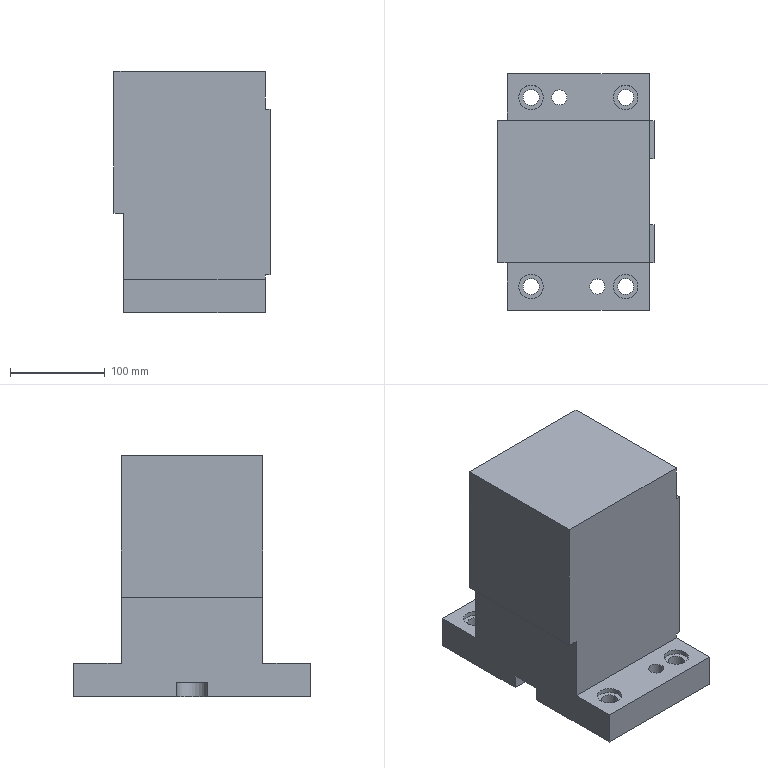Part | NX | features solid 2 | 1 solid | 44 faces | box 165 x 250 x 255 mm | volume 5111238 mm3 | plane 33 | cylinder 11 | commonest cylinder face diameters 17 x4 26 x4 16 x2 32 x1
STEP:
#1=CARTESIAN_POINT('',(655.,586.5,-210.));
#2=VERTEX_POINT('',#1);
#3=CARTESIAN_POINT('',(655.,595.,-210.));
#4=DIRECTION('',(0.,0.,1.));
#5=DIRECTION('',(0.,-1.,0.));
#6=AXIS2_PLACEMENT_3D('',#3,#4,#5);
#7=CIRCLE('',#6,8.5);
#8=EDGE_CURVE('',#2,#2,#7,.T.);
#9=ORIENTED_EDGE('',*,*,#8,.T.);
#10=EDGE_LOOP('',(#9));
#11=FACE_BOUND('',#10,.T.);
#12=CARTESIAN_POINT('',(655.,786.5,-210.));
#13=VERTEX_POINT('',#12);
#14=CARTESIAN_POINT('',(655.,795.,-210.));
#15=DIRECTION('',(0.,0.,1.));
#16=DIRECTION('',(0.,-1.,0.));
#17=AXIS2_PLACEMENT_3D('',#14,#15,#16);
#18=CIRCLE('',#17,8.5);
#19=EDGE_CURVE('',#13,#13,#18,.T.);
#20=ORIENTED_EDGE('',*,*,#19,.T.);
#21=EDGE_LOOP('',(#20));
#22=FACE_BOUND('',#21,.T.);
#23=CARTESIAN_POINT('',(685.,787.,-210.));
#24=VERTEX_POINT('',#23);
#25=CARTESIAN_POINT('',(685.,795.,-210.));
#26=DIRECTION('',(0.,0.,1.));
#27=DIRECTION('',(0.,-1.,0.));
#28=AXIS2_PLACEMENT_3D('',#25,#26,#27);
#29=CIRCLE('',#28,8.);
#30=EDGE_CURVE('',#24,#24,#29,.T.);
#31=ORIENTED_EDGE('',*,*,#30,.T.);
#32=EDGE_LOOP('',(#31));
#33=FACE_BOUND('',#32,.T.);
#34=CARTESIAN_POINT('',(755.,786.5,-210.));
#35=VERTEX_POINT('',#34);
#36=CARTESIAN_POINT('',(755.,795.,-210.));
#37=DIRECTION('',(0.,0.,1.));
#38=DIRECTION('',(0.,-1.,0.));
#39=AXIS2_PLACEMENT_3D('',#36,#37,#38);
#40=CIRCLE('',#39,8.5);
#41=EDGE_CURVE('',#35,#35,#40,.T.);
#42=ORIENTED_EDGE('',*,*,#41,.T.);
#43=EDGE_LOOP('',(#42));
#44=FACE_BOUND('',#43,.T.);
#45=CARTESIAN_POINT('',(725.,587.,-210.));
#46=VERTEX_POINT('',#45);
#47=CARTESIAN_POINT('',(725.,595.,-210.));
#48=DIRECTION('',(0.,0.,1.));
#49=DIRECTION('',(0.,-1.,0.));
#50=AXIS2_PLACEMENT_3D('',#47,#48,#49);
#51=CIRCLE('',#50,8.);
#52=EDGE_CURVE('',#46,#46,#51,.T.);
#53=ORIENTED_EDGE('',*,*,#52,.T.);
#54=EDGE_LOOP('',(#53));
#55=FACE_BOUND('',#54,.T.);
#56=CARTESIAN_POINT('',(755.,586.5,-210.));
#57=VERTEX_POINT('',#56);
#58=CARTESIAN_POINT('',(755.,595.,-210.));
#59=DIRECTION('',(0.,0.,1.));
#60=DIRECTION('',(0.,-1.,0.));
#61=AXIS2_PLACEMENT_3D('',#58,#59,#60);
#62=CIRCLE('',#61,8.5);
#63=EDGE_CURVE('',#57,#57,#62,.T.);
#64=ORIENTED_EDGE('',*,*,#63,.T.);
#65=EDGE_LOOP('',(#64));
#66=FACE_BOUND('',#65,.T.);
#67=CARTESIAN_POINT('',(714.,679.031,-210.));
#68=VERTEX_POINT('',#67);
#69=CARTESIAN_POINT('',(714.,679.,-210.));
#70=VERTEX_POINT('',#69);
#71=CARTESIAN_POINT('',(714.,810.,-210.));
#72=DIRECTION('',(0.,-1.,0.));
#73=VECTOR('',#72,1000.);
#74=LINE('',#71,#73);
#75=EDGE_CURVE('',#68,#70,#74,.T.);
#76=ORIENTED_EDGE('',*,*,#75,.F.);
#77=CARTESIAN_POINT('',(714.,710.969,-210.));
#78=VERTEX_POINT('',#77);
#79=CARTESIAN_POINT('',(715.,695.,-210.));
#80=DIRECTION('',(0.,0.,-1.));
#81=DIRECTION('',(-1.,0.,0.));
#82=AXIS2_PLACEMENT_3D('',#79,#80,#81);
#83=CIRCLE('',#82,16.);
#84=EDGE_CURVE('',#68,#78,#83,.F.);
#85=ORIENTED_EDGE('',*,*,#84,.T.);
#86=CARTESIAN_POINT('',(714.,711.,-210.));
#87=VERTEX_POINT('',#86);
#88=CARTESIAN_POINT('',(714.,810.,-210.));
#89=DIRECTION('',(0.,-1.,0.));
#90=VECTOR('',#89,1000.);
#91=LINE('',#88,#90);
#92=EDGE_CURVE('',#87,#78,#91,.T.);
#93=ORIENTED_EDGE('',*,*,#92,.F.);
#94=CARTESIAN_POINT('',(630.,711.,-210.));
#95=VERTEX_POINT('',#94);
#96=CARTESIAN_POINT('',(780.,711.,-210.));
#97=DIRECTION('',(-1.,0.,0.));
#98=VECTOR('',#97,1000.);
#99=LINE('',#96,#98);
#100=EDGE_CURVE('',#87,#95,#99,.T.);
#101=ORIENTED_EDGE('',*,*,#100,.T.);
#102=CARTESIAN_POINT('',(630.,820.,-210.));
#103=VERTEX_POINT('',#102);
#104=CARTESIAN_POINT('',(630.,810.,-210.));
#105=DIRECTION('',(0.,1.,0.));
#106=VECTOR('',#105,1000.);
#107=LINE('',#104,#106);
#108=EDGE_CURVE('',#103,#95,#107,.F.);
#109=ORIENTED_EDGE('',*,*,#108,.F.);
#110=CARTESIAN_POINT('',(780.,820.,-210.));
#111=VERTEX_POINT('',#110);
#112=CARTESIAN_POINT('',(780.,820.,-210.));
#113=DIRECTION('',(1.,0.,0.));
#114=VECTOR('',#113,1000.);
#115=LINE('',#112,#114);
#116=EDGE_CURVE('',#111,#103,#115,.F.);
#117=ORIENTED_EDGE('',*,*,#116,.F.);
#118=CARTESIAN_POINT('',(780.,570.,-210.));
#119=VERTEX_POINT('',#118);
#120=CARTESIAN_POINT('',(780.,810.,-210.));
#121=DIRECTION('',(0.,-1.,0.));
#122=VECTOR('',#121,1000.);
#123=LINE('',#120,#122);
#124=EDGE_CURVE('',#111,#119,#123,.T.);
#125=ORIENTED_EDGE('',*,*,#124,.T.);
#126=CARTESIAN_POINT('',(630.,570.,-210.));
#127=VERTEX_POINT('',#126);
#128=CARTESIAN_POINT('',(780.,570.,-210.));
#129=DIRECTION('',(1.,0.,0.));
#130=VECTOR('',#129,1000.);
#131=LINE('',#128,#130);
#132=EDGE_CURVE('',#119,#127,#131,.F.);
#133=ORIENTED_EDGE('',*,*,#132,.T.);
#134=CARTESIAN_POINT('',(630.,679.,-210.));
#135=VERTEX_POINT('',#134);
#136=CARTESIAN_POINT('',(630.,810.,-210.));
#137=DIRECTION('',(0.,1.,0.));
#138=VECTOR('',#137,1000.);
#139=LINE('',#136,#138);
#140=EDGE_CURVE('',#135,#127,#139,.F.);
#141=ORIENTED_EDGE('',*,*,#140,.F.);
#142=CARTESIAN_POINT('',(780.,679.,-210.));
#143=DIRECTION('',(1.,0.,0.));
#144=VECTOR('',#143,1000.);
#145=LINE('',#142,#144);
#146=EDGE_CURVE('',#135,#70,#145,.T.);
#147=ORIENTED_EDGE('',*,*,#146,.T.);
#148=EDGE_LOOP('',(#76,#85,#93,#101,#109,#117,#125,#133,#141,#147));
#149=FACE_BOUND('',#148,.T.);
#150=CARTESIAN_POINT('',(780.,810.,-210.));
#151=DIRECTION('',(0.,0.,-1.));
#152=DIRECTION('',(0.,1.,0.));
#153=AXIS2_PLACEMENT_3D('',#150,#151,#152);
#154=PLANE('',#153);
#155=ADVANCED_FACE('',(#11,#22,#33,#44,#55,#66,#149),#154,.T.);
#156=CARTESIAN_POINT('',(714.,679.031,-195.));
#157=VERTEX_POINT('',#156);
#158=CARTESIAN_POINT('',(714.,679.031,-195.));
#159=DIRECTION('',(0.,0.,-1.));
#160=VECTOR('',#159,1000.);
#161=LINE('',#158,#160);
#162=EDGE_CURVE('',#68,#157,#161,.F.);
#163=ORIENTED_EDGE('',*,*,#162,.F.);
#164=ORIENTED_EDGE('',*,*,#75,.T.);
#165=CARTESIAN_POINT('',(714.,679.,-195.));
#166=VERTEX_POINT('',#165);
#167=CARTESIAN_POINT('',(714.,679.,-195.));
#168=DIRECTION('',(0.,0.,-1.));
#169=VECTOR('',#168,1000.);
#170=LINE('',#167,#169);
#171=EDGE_CURVE('',#166,#70,#170,.T.);
#172=ORIENTED_EDGE('',*,*,#171,.F.);
#173=CARTESIAN_POINT('',(714.,650.,-195.));
#174=DIRECTION('',(0.,-1.,0.));
#175=VECTOR('',#174,1000.);
#176=LINE('',#173,#175);
#177=EDGE_CURVE('',#157,#166,#176,.T.);
#178=ORIENTED_EDGE('',*,*,#177,.F.);
#179=EDGE_LOOP('',(#163,#164,#172,#178));
#180=FACE_BOUND('',#179,.T.);
#181=CARTESIAN_POINT('',(714.,810.,-180.));
#182=DIRECTION('',(1.,0.,0.));
#183=DIRECTION('',(0.,0.,-1.));
#184=AXIS2_PLACEMENT_3D('',#181,#182,#183);
#185=PLANE('',#184);
#186=ADVANCED_FACE('',(#180),#185,.F.);
#187=CARTESIAN_POINT('',(714.,710.969,-195.));
#188=VERTEX_POINT('',#187);
#189=CARTESIAN_POINT('',(714.,710.969,-195.));
#190=DIRECTION('',(0.,0.,-1.));
#191=VECTOR('',#190,1000.);
#192=LINE('',#189,#191);
#193=EDGE_CURVE('',#188,#78,#192,.T.);
#194=ORIENTED_EDGE('',*,*,#193,.F.);
#195=CARTESIAN_POINT('',(714.,711.,-195.));
#196=VERTEX_POINT('',#195);
#197=CARTESIAN_POINT('',(714.,650.,-195.));
#198=DIRECTION('',(0.,-1.,0.));
#199=VECTOR('',#198,1000.);
#200=LINE('',#197,#199);
#201=EDGE_CURVE('',#196,#188,#200,.T.);
#202=ORIENTED_EDGE('',*,*,#201,.F.);
#203=CARTESIAN_POINT('',(714.,711.,-180.));
#204=DIRECTION('',(0.,0.,-1.));
#205=VECTOR('',#204,1000.);
#206=LINE('',#203,#205);
#207=EDGE_CURVE('',#196,#87,#206,.T.);
#208=ORIENTED_EDGE('',*,*,#207,.T.);
#209=ORIENTED_EDGE('',*,*,#92,.T.);
#210=EDGE_LOOP('',(#194,#202,#208,#209));
#211=FACE_BOUND('',#210,.T.);
#212=CARTESIAN_POINT('',(714.,810.,-180.));
#213=DIRECTION('',(1.,0.,0.));
#214=DIRECTION('',(0.,0.,-1.));
#215=AXIS2_PLACEMENT_3D('',#212,#213,#214);
#216=PLANE('',#215);
#217=ADVANCED_FACE('',(#211),#216,.F.);
#218=CARTESIAN_POINT('',(715.,695.,-195.));
#219=DIRECTION('',(0.,0.,-1.));
#220=DIRECTION('',(-1.,0.,0.));
#221=AXIS2_PLACEMENT_3D('',#218,#219,#220);
#222=CIRCLE('',#221,16.);
#223=EDGE_CURVE('',#157,#188,#222,.F.);
#224=ORIENTED_EDGE('',*,*,#223,.F.);
#225=ORIENTED_EDGE('',*,*,#177,.T.);
#226=CARTESIAN_POINT('',(630.,679.,-195.));
#227=VERTEX_POINT('',#226);
#228=CARTESIAN_POINT('',(740.,679.,-195.));
#229=DIRECTION('',(-1.,0.,0.));
#230=VECTOR('',#229,1000.);
#231=LINE('',#228,#230);
#232=EDGE_CURVE('',#227,#166,#231,.F.);
#233=ORIENTED_EDGE('',*,*,#232,.F.);
#234=CARTESIAN_POINT('',(630.,711.,-195.));
#235=VERTEX_POINT('',#234);
#236=CARTESIAN_POINT('',(630.,810.,-195.));
#237=DIRECTION('',(0.,1.,0.));
#238=VECTOR('',#237,1000.);
#239=LINE('',#236,#238);
#240=EDGE_CURVE('',#235,#227,#239,.F.);
#241=ORIENTED_EDGE('',*,*,#240,.F.);
#242=CARTESIAN_POINT('',(740.,711.,-195.));
#243=DIRECTION('',(1.,0.,0.));
#244=VECTOR('',#243,1000.);
#245=LINE('',#242,#244);
#246=EDGE_CURVE('',#196,#235,#245,.F.);
#247=ORIENTED_EDGE('',*,*,#246,.F.);
#248=ORIENTED_EDGE('',*,*,#201,.T.);
#249=EDGE_LOOP('',(#224,#225,#233,#241,#247,#248));
#250=FACE_BOUND('',#249,.T.);
#251=CARTESIAN_POINT('',(740.,650.,-195.));
#252=DIRECTION('',(0.,0.,-1.));
#253=DIRECTION('',(-1.,0.,0.));
#254=AXIS2_PLACEMENT_3D('',#251,#252,#253);
#255=PLANE('',#254);
#256=ADVANCED_FACE('',(#250),#255,.T.);
#257=CARTESIAN_POINT('',(780.,730.,5.));
#258=VERTEX_POINT('',#257);
#259=CARTESIAN_POINT('',(780.,770.,5.));
#260=VERTEX_POINT('',#259);
#261=CARTESIAN_POINT('',(780.,730.,5.));
#262=DIRECTION('',(0.,1.,0.));
#263=VECTOR('',#262,1000.);
#264=LINE('',#261,#263);
#265=EDGE_CURVE('',#258,#260,#264,.T.);
#266=ORIENTED_EDGE('',*,*,#265,.T.);
#267=CARTESIAN_POINT('',(780.,770.,45.));
#268=VERTEX_POINT('',#267);
#269=CARTESIAN_POINT('',(780.,770.,-220.));
#270=DIRECTION('',(0.,0.,-1.));
#271=VECTOR('',#270,1000.);
#272=LINE('',#269,#271);
#273=EDGE_CURVE('',#260,#268,#272,.F.);
#274=ORIENTED_EDGE('',*,*,#273,.T.);
#275=CARTESIAN_POINT('',(780.,620.,45.));
#276=VERTEX_POINT('',#275);
#277=CARTESIAN_POINT('',(780.,810.,45.));
#278=DIRECTION('',(0.,-1.,0.));
#279=VECTOR('',#278,1000.);
#280=LINE('',#277,#279);
#281=EDGE_CURVE('',#268,#276,#280,.T.);
#282=ORIENTED_EDGE('',*,*,#281,.T.);
#283=CARTESIAN_POINT('',(780.,620.,5.));
#284=VERTEX_POINT('',#283);
#285=CARTESIAN_POINT('',(780.,620.,-220.));
#286=DIRECTION('',(0.,0.,1.));
#287=VECTOR('',#286,1000.);
#288=LINE('',#285,#287);
#289=EDGE_CURVE('',#284,#276,#288,.T.);
#290=ORIENTED_EDGE('',*,*,#289,.F.);
#291=CARTESIAN_POINT('',(780.,660.,5.));
#292=VERTEX_POINT('',#291);
#293=CARTESIAN_POINT('',(780.,620.,5.));
#294=DIRECTION('',(0.,1.,0.));
#295=VECTOR('',#294,1000.);
#296=LINE('',#293,#295);
#297=EDGE_CURVE('',#284,#292,#296,.T.);
#298=ORIENTED_EDGE('',*,*,#297,.T.);
#299=CARTESIAN_POINT('',(780.,810.,5.));
#300=DIRECTION('',(0.,-1.,0.));
#301=VECTOR('',#300,1000.);
#302=LINE('',#299,#301);
#303=EDGE_CURVE('',#258,#292,#302,.T.);
#304=ORIENTED_EDGE('',*,*,#303,.F.);
#305=EDGE_LOOP('',(#266,#274,#282,#290,#298,#304));
#306=FACE_BOUND('',#305,.T.);
#307=CARTESIAN_POINT('',(780.,810.,-220.));
#308=DIRECTION('',(1.,0.,0.));
#309=DIRECTION('',(0.,-1.,0.));
#310=AXIS2_PLACEMENT_3D('',#307,#308,#309);
#311=PLANE('',#310);
#312=ADVANCED_FACE('',(#306),#311,.T.);
#313=ORIENTED_EDGE('',*,*,#108,.T.);
#314=CARTESIAN_POINT('',(630.,711.,-220.));
#315=DIRECTION('',(0.,0.,-1.));
#316=VECTOR('',#315,1000.);
#317=LINE('',#314,#316);
#318=EDGE_CURVE('',#95,#235,#317,.F.);
#319=ORIENTED_EDGE('',*,*,#318,.T.);
#320=ORIENTED_EDGE('',*,*,#240,.T.);
#321=CARTESIAN_POINT('',(630.,679.,-220.));
#322=DIRECTION('',(0.,0.,1.));
#323=VECTOR('',#322,1000.);
#324=LINE('',#321,#323);
#325=EDGE_CURVE('',#227,#135,#324,.F.);
#326=ORIENTED_EDGE('',*,*,#325,.T.);
#327=ORIENTED_EDGE('',*,*,#140,.T.);
#328=CARTESIAN_POINT('',(630.,570.,-175.));
#329=VERTEX_POINT('',#328);
#330=CARTESIAN_POINT('',(630.,570.,-180.));
#331=DIRECTION('',(0.,0.,-1.));
#332=VECTOR('',#331,1000.);
#333=LINE('',#330,#332);
#334=EDGE_CURVE('',#329,#127,#333,.T.);
#335=ORIENTED_EDGE('',*,*,#334,.F.);
#336=CARTESIAN_POINT('',(630.,620.,-175.));
#337=VERTEX_POINT('',#336);
#338=CARTESIAN_POINT('',(630.,810.,-175.));
#339=DIRECTION('',(0.,-1.,0.));
#340=VECTOR('',#339,1000.);
#341=LINE('',#338,#340);
#342=EDGE_CURVE('',#337,#329,#341,.T.);
#343=ORIENTED_EDGE('',*,*,#342,.F.);
#344=CARTESIAN_POINT('',(630.,620.,-105.));
#345=VERTEX_POINT('',#344);
#346=CARTESIAN_POINT('',(630.,620.,-220.));
#347=DIRECTION('',(0.,0.,-1.));
#348=VECTOR('',#347,1000.);
#349=LINE('',#346,#348);
#350=EDGE_CURVE('',#337,#345,#349,.F.);
#351=ORIENTED_EDGE('',*,*,#350,.T.);
#352=CARTESIAN_POINT('',(630.,770.,-105.));
#353=VERTEX_POINT('',#352);
#354=CARTESIAN_POINT('',(630.,770.,-105.));
#355=DIRECTION('',(0.,1.,0.));
#356=VECTOR('',#355,1000.);
#357=LINE('',#354,#356);
#358=EDGE_CURVE('',#353,#345,#357,.F.);
#359=ORIENTED_EDGE('',*,*,#358,.F.);
#360=CARTESIAN_POINT('',(630.,770.,-175.));
#361=VERTEX_POINT('',#360);
#362=CARTESIAN_POINT('',(630.,770.,-220.));
#363=DIRECTION('',(0.,0.,1.));
#364=VECTOR('',#363,1000.);
#365=LINE('',#362,#364);
#366=EDGE_CURVE('',#361,#353,#365,.T.);
#367=ORIENTED_EDGE('',*,*,#366,.F.);
#368=CARTESIAN_POINT('',(630.,820.,-175.));
#369=VERTEX_POINT('',#368);
#370=CARTESIAN_POINT('',(630.,810.,-175.));
#371=DIRECTION('',(0.,-1.,0.));
#372=VECTOR('',#371,1000.);
#373=LINE('',#370,#372);
#374=EDGE_CURVE('',#361,#369,#373,.F.);
#375=ORIENTED_EDGE('',*,*,#374,.T.);
#376=CARTESIAN_POINT('',(630.,820.,-180.));
#377=DIRECTION('',(0.,0.,-1.));
#378=VECTOR('',#377,1000.);
#379=LINE('',#376,#378);
#380=EDGE_CURVE('',#369,#103,#379,.T.);
#381=ORIENTED_EDGE('',*,*,#380,.T.);
#382=EDGE_LOOP('',(#313,#319,#320,#326,#327,#335,#343,#351,#359,#367,#375,#381));
#383=FACE_BOUND('',#382,.T.);
#384=CARTESIAN_POINT('',(630.,810.,-220.));
#385=DIRECTION('',(1.,0.,0.));
#386=DIRECTION('',(0.,-1.,0.));
#387=AXIS2_PLACEMENT_3D('',#384,#385,#386);
#388=PLANE('',#387);
#389=ADVANCED_FACE('',(#383),#388,.F.);
#390=CARTESIAN_POINT('',(780.,730.,-170.));
#391=VERTEX_POINT('',#390);
#392=CARTESIAN_POINT('',(780.,770.,-170.));
#393=VERTEX_POINT('',#392);
#394=CARTESIAN_POINT('',(780.,730.,-170.));
#395=DIRECTION('',(0.,1.,0.));
#396=VECTOR('',#395,1000.);
#397=LINE('',#394,#396);
#398=EDGE_CURVE('',#391,#393,#397,.T.);
#399=ORIENTED_EDGE('',*,*,#398,.F.);
#400=CARTESIAN_POINT('',(780.,660.,-170.));
#401=VERTEX_POINT('',#400);
#402=CARTESIAN_POINT('',(780.,810.,-170.));
#403=DIRECTION('',(0.,-1.,0.));
#404=VECTOR('',#403,1000.);
#405=LINE('',#402,#404);
#406=EDGE_CURVE('',#391,#401,#405,.T.);
#407=ORIENTED_EDGE('',*,*,#406,.T.);
#408=CARTESIAN_POINT('',(780.,620.,-170.));
#409=VERTEX_POINT('',#408);
#410=CARTESIAN_POINT('',(780.,620.,-170.));
#411=DIRECTION('',(0.,1.,0.));
#412=VECTOR('',#411,1000.);
#413=LINE('',#410,#412);
#414=EDGE_CURVE('',#409,#401,#413,.T.);
#415=ORIENTED_EDGE('',*,*,#414,.F.);
#416=CARTESIAN_POINT('',(780.,620.,-175.));
#417=VERTEX_POINT('',#416);
#418=CARTESIAN_POINT('',(780.,620.,-220.));
#419=DIRECTION('',(0.,0.,1.));
#420=VECTOR('',#419,1000.);
#421=LINE('',#418,#420);
#422=EDGE_CURVE('',#417,#409,#421,.T.);
#423=ORIENTED_EDGE('',*,*,#422,.F.);
#424=CARTESIAN_POINT('',(780.,570.,-175.));
#425=VERTEX_POINT('',#424);
#426=CARTESIAN_POINT('',(780.,620.,-175.));
#427=DIRECTION('',(0.,1.,0.));
#428=VECTOR('',#427,1000.);
#429=LINE('',#426,#428);
#430=EDGE_CURVE('',#417,#425,#429,.F.);
#431=ORIENTED_EDGE('',*,*,#430,.T.);
#432=CARTESIAN_POINT('',(780.,570.,-180.));
#433=DIRECTION('',(0.,0.,-1.));
#434=VECTOR('',#433,1000.);
#435=LINE('',#432,#434);
#436=EDGE_CURVE('',#425,#119,#435,.T.);
#437=ORIENTED_EDGE('',*,*,#436,.T.);
#438=ORIENTED_EDGE('',*,*,#124,.F.);
#439=CARTESIAN_POINT('',(780.,820.,-175.));
#440=VERTEX_POINT('',#439);
#441=CARTESIAN_POINT('',(780.,820.,-180.));
#442=DIRECTION('',(0.,0.,1.));
#443=VECTOR('',#442,1000.);
#444=LINE('',#441,#443);
#445=EDGE_CURVE('',#440,#111,#444,.F.);
#446=ORIENTED_EDGE('',*,*,#445,.F.);
#447=CARTESIAN_POINT('',(780.,770.,-175.));
#448=VERTEX_POINT('',#447);
#449=CARTESIAN_POINT('',(780.,770.,-175.));
#450=DIRECTION('',(0.,1.,0.));
#451=VECTOR('',#450,1000.);
#452=LINE('',#449,#451);
#453=EDGE_CURVE('',#448,#440,#452,.T.);
#454=ORIENTED_EDGE('',*,*,#453,.F.);
#455=CARTESIAN_POINT('',(780.,770.,-220.));
#456=DIRECTION('',(0.,0.,-1.));
#457=VECTOR('',#456,1000.);
#458=LINE('',#455,#457);
#459=EDGE_CURVE('',#448,#393,#458,.F.);
#460=ORIENTED_EDGE('',*,*,#459,.T.);
#461=EDGE_LOOP('',(#399,#407,#415,#423,#431,#437,#438,#446,#454,#460));
#462=FACE_BOUND('',#461,.T.);
#463=CARTESIAN_POINT('',(780.,810.,-220.));
#464=DIRECTION('',(1.,0.,0.));
#465=DIRECTION('',(0.,-1.,0.));
#466=AXIS2_PLACEMENT_3D('',#463,#464,#465);
#467=PLANE('',#466);
#468=ADVANCED_FACE('',(#462),#467,.T.);
#469=ORIENTED_EDGE('',*,*,#459,.F.);
#470=CARTESIAN_POINT('',(780.,770.,-175.));
#471=DIRECTION('',(1.,0.,0.));
#472=VECTOR('',#471,1000.);
#473=LINE('',#470,#472);
#474=EDGE_CURVE('',#448,#361,#473,.F.);
#475=ORIENTED_EDGE('',*,*,#474,.T.);
#476=ORIENTED_EDGE('',*,*,#366,.T.);
#477=CARTESIAN_POINT('',(620.,770.,-105.));
#478=VERTEX_POINT('',#477);
#479=CARTESIAN_POINT('',(630.,770.,-105.));
#480=DIRECTION('',(1.,0.,0.));
#481=VECTOR('',#480,1000.);
#482=LINE('',#479,#481);
#483=EDGE_CURVE('',#353,#478,#482,.F.);
#484=ORIENTED_EDGE('',*,*,#483,.T.);
#485=CARTESIAN_POINT('',(620.,770.,45.));
#486=VERTEX_POINT('',#485);
#487=CARTESIAN_POINT('',(620.,770.,45.));
#488=DIRECTION('',(0.,0.,1.));
#489=VECTOR('',#488,1000.);
#490=LINE('',#487,#489);
#491=EDGE_CURVE('',#486,#478,#490,.F.);
#492=ORIENTED_EDGE('',*,*,#491,.F.);
#493=CARTESIAN_POINT('',(780.,770.,45.));
#494=DIRECTION('',(1.,0.,0.));
#495=VECTOR('',#494,1000.);
#496=LINE('',#493,#495);
#497=EDGE_CURVE('',#268,#486,#496,.F.);
#498=ORIENTED_EDGE('',*,*,#497,.F.);
#499=ORIENTED_EDGE('',*,*,#273,.F.);
#500=CARTESIAN_POINT('',(785.,770.,5.));
#501=VERTEX_POINT('',#500);
#502=CARTESIAN_POINT('',(780.,770.,5.));
#503=DIRECTION('',(1.,0.,0.));
#504=VECTOR('',#503,1000.);
#505=LINE('',#502,#504);
#506=EDGE_CURVE('',#260,#501,#505,.T.);
#507=ORIENTED_EDGE('',*,*,#506,.T.);
#508=CARTESIAN_POINT('',(785.,770.,-170.));
#509=VERTEX_POINT('',#508);
#510=CARTESIAN_POINT('',(785.,770.,-170.));
#511=DIRECTION('',(0.,0.,-1.));
#512=VECTOR('',#511,1000.);
#513=LINE('',#510,#512);
#514=EDGE_CURVE('',#501,#509,#513,.T.);
#515=ORIENTED_EDGE('',*,*,#514,.T.);
#516=CARTESIAN_POINT('',(780.,770.,-170.));
#517=DIRECTION('',(1.,0.,0.));
#518=VECTOR('',#517,1000.);
#519=LINE('',#516,#518);
#520=EDGE_CURVE('',#393,#509,#519,.T.);
#521=ORIENTED_EDGE('',*,*,#520,.F.);
#522=EDGE_LOOP('',(#469,#475,#476,#484,#492,#498,#499,#507,#515,#521));
#523=FACE_BOUND('',#522,.T.);
#524=CARTESIAN_POINT('',(780.,770.,-220.));
#525=DIRECTION('',(0.,-1.,0.));
#526=DIRECTION('',(-1.,0.,0.));
#527=AXIS2_PLACEMENT_3D('',#524,#525,#526);
#528=PLANE('',#527);
#529=ADVANCED_FACE('',(#523),#528,.F.);
#530=ORIENTED_EDGE('',*,*,#497,.T.);
#531=CARTESIAN_POINT('',(620.,620.,45.));
#532=VERTEX_POINT('',#531);
#533=CARTESIAN_POINT('',(620.,770.,45.));
#534=DIRECTION('',(0.,-1.,0.));
#535=VECTOR('',#534,1000.);
#536=LINE('',#533,#535);
#537=EDGE_CURVE('',#486,#532,#536,.T.);
#538=ORIENTED_EDGE('',*,*,#537,.T.);
#539=CARTESIAN_POINT('',(780.,620.,45.));
#540=DIRECTION('',(-1.,0.,0.));
#541=VECTOR('',#540,1000.);
#542=LINE('',#539,#541);
#543=EDGE_CURVE('',#276,#532,#542,.T.);
#544=ORIENTED_EDGE('',*,*,#543,.F.);
#545=ORIENTED_EDGE('',*,*,#281,.F.);
#546=EDGE_LOOP('',(#530,#538,#544,#545));
#547=FACE_BOUND('',#546,.T.);
#548=CARTESIAN_POINT('',(780.,810.,45.));
#549=DIRECTION('',(0.,0.,-1.));
#550=DIRECTION('',(0.,1.,0.));
#551=AXIS2_PLACEMENT_3D('',#548,#549,#550);
#552=PLANE('',#551);
#553=ADVANCED_FACE('',(#547),#552,.F.);
#554=CARTESIAN_POINT('',(780.,620.,-175.));
#555=DIRECTION('',(1.,0.,0.));
#556=VECTOR('',#555,1000.);
#557=LINE('',#554,#556);
#558=EDGE_CURVE('',#417,#337,#557,.F.);
#559=ORIENTED_EDGE('',*,*,#558,.F.);
#560=ORIENTED_EDGE('',*,*,#422,.T.);
#561=CARTESIAN_POINT('',(785.,620.,-170.));
#562=VERTEX_POINT('',#561);
#563=CARTESIAN_POINT('',(780.,620.,-170.));
#564=DIRECTION('',(1.,0.,0.));
#565=VECTOR('',#564,1000.);
#566=LINE('',#563,#565);
#567=EDGE_CURVE('',#409,#562,#566,.T.);
#568=ORIENTED_EDGE('',*,*,#567,.T.);
#569=CARTESIAN_POINT('',(785.,620.,5.));
#570=VERTEX_POINT('',#569);
#571=CARTESIAN_POINT('',(785.,620.,-170.));
#572=DIRECTION('',(0.,0.,-1.));
#573=VECTOR('',#572,1000.);
#574=LINE('',#571,#573);
#575=EDGE_CURVE('',#570,#562,#574,.T.);
#576=ORIENTED_EDGE('',*,*,#575,.F.);
#577=CARTESIAN_POINT('',(780.,620.,5.));
#578=DIRECTION('',(1.,0.,0.));
#579=VECTOR('',#578,1000.);
#580=LINE('',#577,#579);
#581=EDGE_CURVE('',#284,#570,#580,.T.);
#582=ORIENTED_EDGE('',*,*,#581,.F.);
#583=ORIENTED_EDGE('',*,*,#289,.T.);
#584=ORIENTED_EDGE('',*,*,#543,.T.);
#585=CARTESIAN_POINT('',(620.,620.,-105.));
#586=VERTEX_POINT('',#585);
#587=CARTESIAN_POINT('',(620.,620.,45.));
#588=DIRECTION('',(0.,0.,1.));
#589=VECTOR('',#588,1000.);
#590=LINE('',#587,#589);
#591=EDGE_CURVE('',#532,#586,#590,.F.);
#592=ORIENTED_EDGE('',*,*,#591,.T.);
#593=CARTESIAN_POINT('',(630.,620.,-105.));
#594=DIRECTION('',(1.,0.,0.));
#595=VECTOR('',#594,1000.);
#596=LINE('',#593,#595);
#597=EDGE_CURVE('',#345,#586,#596,.F.);
#598=ORIENTED_EDGE('',*,*,#597,.F.);
#599=ORIENTED_EDGE('',*,*,#350,.F.);
#600=EDGE_LOOP('',(#559,#560,#568,#576,#582,#583,#584,#592,#598,#599));
#601=FACE_BOUND('',#600,.T.);
#602=CARTESIAN_POINT('',(780.,620.,-220.));
#603=DIRECTION('',(0.,-1.,0.));
#604=DIRECTION('',(-1.,0.,0.));
#605=AXIS2_PLACEMENT_3D('',#602,#603,#604);
#606=PLANE('',#605);
#607=ADVANCED_FACE('',(#601),#606,.T.);
#608=CARTESIAN_POINT('',(755.,582.,-175.));
#609=VERTEX_POINT('',#608);
#610=CARTESIAN_POINT('',(755.,595.,-175.));
#611=DIRECTION('',(0.,0.,1.));
#612=DIRECTION('',(0.,-1.,0.));
#613=AXIS2_PLACEMENT_3D('',#610,#611,#612);
#614=CIRCLE('',#613,13.);
#615=EDGE_CURVE('',#609,#609,#614,.F.);
#616=ORIENTED_EDGE('',*,*,#615,.T.);
#617=EDGE_LOOP('',(#616));
#618=FACE_BOUND('',#617,.T.);
#619=CARTESIAN_POINT('',(725.,587.,-175.));
#620=VERTEX_POINT('',#619);
#621=CARTESIAN_POINT('',(725.,595.,-175.));
#622=DIRECTION('',(0.,0.,1.));
#623=DIRECTION('',(0.,-1.,0.));
#624=AXIS2_PLACEMENT_3D('',#621,#622,#623);
#625=CIRCLE('',#624,8.);
#626=EDGE_CURVE('',#620,#620,#625,.F.);
#627=ORIENTED_EDGE('',*,*,#626,.T.);
#628=EDGE_LOOP('',(#627));
#629=FACE_BOUND('',#628,.T.);
#630=CARTESIAN_POINT('',(655.,582.,-175.));
#631=VERTEX_POINT('',#630);
#632=CARTESIAN_POINT('',(655.,595.,-175.));
#633=DIRECTION('',(0.,0.,1.));
#634=DIRECTION('',(0.,-1.,0.));
#635=AXIS2_PLACEMENT_3D('',#632,#633,#634);
#636=CIRCLE('',#635,13.);
#637=EDGE_CURVE('',#631,#631,#636,.F.);
#638=ORIENTED_EDGE('',*,*,#637,.T.);
#639=EDGE_LOOP('',(#638));
#640=FACE_BOUND('',#639,.T.);
#641=ORIENTED_EDGE('',*,*,#342,.T.);
#642=CARTESIAN_POINT('',(780.,570.,-175.));
#643=DIRECTION('',(1.,0.,0.));
#644=VECTOR('',#643,1000.);
#645=LINE('',#642,#644);
#646=EDGE_CURVE('',#425,#329,#645,.F.);
#647=ORIENTED_EDGE('',*,*,#646,.F.);
#648=ORIENTED_EDGE('',*,*,#430,.F.);
#649=ORIENTED_EDGE('',*,*,#558,.T.);
#650=EDGE_LOOP('',(#641,#647,#648,#649));
#651=FACE_BOUND('',#650,.T.);
#652=CARTESIAN_POINT('',(780.,620.,-175.));
#653=DIRECTION('',(0.,0.,1.));
#654=DIRECTION('',(-1.,0.,0.));
#655=AXIS2_PLACEMENT_3D('',#652,#653,#654);
#656=PLANE('',#655);
#657=ADVANCED_FACE('',(#618,#629,#640,#651),#656,.T.);
#658=ORIENTED_EDGE('',*,*,#132,.F.);
#659=ORIENTED_EDGE('',*,*,#436,.F.);
#660=ORIENTED_EDGE('',*,*,#646,.T.);
#661=ORIENTED_EDGE('',*,*,#334,.T.);
#662=EDGE_LOOP('',(#658,#659,#660,#661));
#663=FACE_BOUND('',#662,.T.);
#664=CARTESIAN_POINT('',(780.,570.,-180.));
#665=DIRECTION('',(0.,-1.,0.));
#666=DIRECTION('',(0.,0.,-1.));
#667=AXIS2_PLACEMENT_3D('',#664,#665,#666);
#668=PLANE('',#667);
#669=ADVANCED_FACE('',(#663),#668,.T.);
#670=CARTESIAN_POINT('',(755.,782.,-175.));
#671=VERTEX_POINT('',#670);
#672=CARTESIAN_POINT('',(755.,795.,-175.));
#673=DIRECTION('',(0.,0.,1.));
#674=DIRECTION('',(0.,-1.,0.));
#675=AXIS2_PLACEMENT_3D('',#672,#673,#674);
#676=CIRCLE('',#675,13.);
#677=EDGE_CURVE('',#671,#671,#676,.T.);
#678=ORIENTED_EDGE('',*,*,#677,.F.);
#679=EDGE_LOOP('',(#678));
#680=FACE_BOUND('',#679,.T.);
#681=CARTESIAN_POINT('',(685.,787.,-175.));
#682=VERTEX_POINT('',#681);
#683=CARTESIAN_POINT('',(685.,795.,-175.));
#684=DIRECTION('',(0.,0.,1.));
#685=DIRECTION('',(0.,-1.,0.));
#686=AXIS2_PLACEMENT_3D('',#683,#684,#685);
#687=CIRCLE('',#686,8.);
#688=EDGE_CURVE('',#682,#682,#687,.T.);
#689=ORIENTED_EDGE('',*,*,#688,.F.);
#690=EDGE_LOOP('',(#689));
#691=FACE_BOUND('',#690,.T.);
#692=CARTESIAN_POINT('',(655.,782.,-175.));
#693=VERTEX_POINT('',#692);
#694=CARTESIAN_POINT('',(655.,795.,-175.));
#695=DIRECTION('',(0.,0.,1.));
#696=DIRECTION('',(0.,-1.,0.));
#697=AXIS2_PLACEMENT_3D('',#694,#695,#696);
#698=CIRCLE('',#697,13.);
#699=EDGE_CURVE('',#693,#693,#698,.T.);
#700=ORIENTED_EDGE('',*,*,#699,.F.);
#701=EDGE_LOOP('',(#700));
#702=FACE_BOUND('',#701,.T.);
#703=ORIENTED_EDGE('',*,*,#374,.F.);
#704=ORIENTED_EDGE('',*,*,#474,.F.);
#705=ORIENTED_EDGE('',*,*,#453,.T.);
#706=CARTESIAN_POINT('',(780.,820.,-175.));
#707=DIRECTION('',(-1.,0.,0.));
#708=VECTOR('',#707,1000.);
#709=LINE('',#706,#708);
#710=EDGE_CURVE('',#440,#369,#709,.T.);
#711=ORIENTED_EDGE('',*,*,#710,.T.);
#712=EDGE_LOOP('',(#703,#704,#705,#711));
#713=FACE_BOUND('',#712,.T.);
#714=CARTESIAN_POINT('',(780.,770.,-175.));
#715=DIRECTION('',(0.,0.,1.));
#716=DIRECTION('',(-1.,0.,0.));
#717=AXIS2_PLACEMENT_3D('',#714,#715,#716);
#718=PLANE('',#717);
#719=ADVANCED_FACE('',(#680,#691,#702,#713),#718,.T.);
#720=ORIENTED_EDGE('',*,*,#116,.T.);
#721=ORIENTED_EDGE('',*,*,#380,.F.);
#722=ORIENTED_EDGE('',*,*,#710,.F.);
#723=ORIENTED_EDGE('',*,*,#445,.T.);
#724=EDGE_LOOP('',(#720,#721,#722,#723));
#725=FACE_BOUND('',#724,.T.);
#726=CARTESIAN_POINT('',(780.,820.,-180.));
#727=DIRECTION('',(0.,-1.,0.));
#728=DIRECTION('',(0.,0.,-1.));
#729=AXIS2_PLACEMENT_3D('',#726,#727,#728);
#730=PLANE('',#729);
#731=ADVANCED_FACE('',(#725),#730,.F.);
#732=CARTESIAN_POINT('',(670.,730.,-170.));
#733=VERTEX_POINT('',#732);
#734=CARTESIAN_POINT('',(780.,730.,-170.));
#735=DIRECTION('',(1.,0.,0.));
#736=VECTOR('',#735,1000.);
#737=LINE('',#734,#736);
#738=EDGE_CURVE('',#391,#733,#737,.F.);
#739=ORIENTED_EDGE('',*,*,#738,.F.);
#740=CARTESIAN_POINT('',(785.,730.,-170.));
#741=VERTEX_POINT('',#740);
#742=CARTESIAN_POINT('',(780.,730.,-170.));
#743=DIRECTION('',(1.,0.,0.));
#744=VECTOR('',#743,1000.);
#745=LINE('',#742,#744);
#746=EDGE_CURVE('',#391,#741,#745,.T.);
#747=ORIENTED_EDGE('',*,*,#746,.T.);
#748=CARTESIAN_POINT('',(785.,730.,5.));
#749=VERTEX_POINT('',#748);
#750=CARTESIAN_POINT('',(785.,730.,-170.));
#751=DIRECTION('',(0.,0.,-1.));
#752=VECTOR('',#751,1000.);
#753=LINE('',#750,#752);
#754=EDGE_CURVE('',#749,#741,#753,.T.);
#755=ORIENTED_EDGE('',*,*,#754,.F.);
#756=CARTESIAN_POINT('',(780.,730.,5.));
#757=DIRECTION('',(1.,0.,0.));
#758=VECTOR('',#757,1000.);
#759=LINE('',#756,#758);
#760=EDGE_CURVE('',#258,#749,#759,.T.);
#761=ORIENTED_EDGE('',*,*,#760,.F.);
#762=CARTESIAN_POINT('',(670.,730.,5.));
#763=VERTEX_POINT('',#762);
#764=CARTESIAN_POINT('',(780.,730.,5.));
#765=DIRECTION('',(1.,0.,0.));
#766=VECTOR('',#765,1000.);
#767=LINE('',#764,#766);
#768=EDGE_CURVE('',#258,#763,#767,.F.);
#769=ORIENTED_EDGE('',*,*,#768,.T.);
#770=CARTESIAN_POINT('',(670.,730.,-220.));
#771=DIRECTION('',(0.,0.,1.));
#772=VECTOR('',#771,1000.);
#773=LINE('',#770,#772);
#774=EDGE_CURVE('',#733,#763,#773,.T.);
#775=ORIENTED_EDGE('',*,*,#774,.F.);
#776=EDGE_LOOP('',(#739,#747,#755,#761,#769,#775));
#777=FACE_BOUND('',#776,.T.);
#778=CARTESIAN_POINT('',(780.,730.,-220.));
#779=DIRECTION('',(0.,-1.,0.));
#780=DIRECTION('',(-1.,0.,0.));
#781=AXIS2_PLACEMENT_3D('',#778,#779,#780);
#782=PLANE('',#781);
#783=ADVANCED_FACE('',(#777),#782,.T.);
#784=ORIENTED_EDGE('',*,*,#774,.T.);
#785=CARTESIAN_POINT('',(670.,660.,5.));
#786=VERTEX_POINT('',#785);
#787=CARTESIAN_POINT('',(670.,810.,5.));
#788=DIRECTION('',(0.,1.,0.));
#789=VECTOR('',#788,1000.);
#790=LINE('',#787,#789);
#791=EDGE_CURVE('',#763,#786,#790,.F.);
#792=ORIENTED_EDGE('',*,*,#791,.T.);
#793=CARTESIAN_POINT('',(670.,660.,-170.));
#794=VERTEX_POINT('',#793);
#795=CARTESIAN_POINT('',(670.,660.,-220.));
#796=DIRECTION('',(0.,0.,-1.));
#797=VECTOR('',#796,1000.);
#798=LINE('',#795,#797);
#799=EDGE_CURVE('',#794,#786,#798,.F.);
#800=ORIENTED_EDGE('',*,*,#799,.F.);
#801=CARTESIAN_POINT('',(670.,810.,-170.));
#802=DIRECTION('',(0.,1.,0.));
#803=VECTOR('',#802,1000.);
#804=LINE('',#801,#803);
#805=EDGE_CURVE('',#733,#794,#804,.F.);
#806=ORIENTED_EDGE('',*,*,#805,.F.);
#807=EDGE_LOOP('',(#784,#792,#800,#806));
#808=FACE_BOUND('',#807,.T.);
#809=CARTESIAN_POINT('',(670.,810.,-220.));
#810=DIRECTION('',(1.,0.,0.));
#811=DIRECTION('',(0.,-1.,0.));
#812=AXIS2_PLACEMENT_3D('',#809,#810,#811);
#813=PLANE('',#812);
#814=ADVANCED_FACE('',(#808),#813,.T.);
#815=ORIENTED_EDGE('',*,*,#791,.F.);
#816=ORIENTED_EDGE('',*,*,#768,.F.);
#817=ORIENTED_EDGE('',*,*,#303,.T.);
#818=CARTESIAN_POINT('',(780.,660.,5.));
#819=DIRECTION('',(-1.,0.,0.));
#820=VECTOR('',#819,1000.);
#821=LINE('',#818,#820);
#822=EDGE_CURVE('',#292,#786,#821,.T.);
#823=ORIENTED_EDGE('',*,*,#822,.T.);
#824=EDGE_LOOP('',(#815,#816,#817,#823));
#825=FACE_BOUND('',#824,.T.);
#826=CARTESIAN_POINT('',(780.,810.,5.));
#827=DIRECTION('',(0.,0.,-1.));
#828=DIRECTION('',(0.,1.,0.));
#829=AXIS2_PLACEMENT_3D('',#826,#827,#828);
#830=PLANE('',#829);
#831=ADVANCED_FACE('',(#825),#830,.T.);
#832=CARTESIAN_POINT('',(780.,660.,-170.));
#833=DIRECTION('',(-1.,0.,0.));
#834=VECTOR('',#833,1000.);
#835=LINE('',#832,#834);
#836=EDGE_CURVE('',#401,#794,#835,.T.);
#837=ORIENTED_EDGE('',*,*,#836,.T.);
#838=ORIENTED_EDGE('',*,*,#799,.T.);
#839=ORIENTED_EDGE('',*,*,#822,.F.);
#840=CARTESIAN_POINT('',(785.,660.,5.));
#841=VERTEX_POINT('',#840);
#842=CARTESIAN_POINT('',(780.,660.,5.));
#843=DIRECTION('',(1.,0.,0.));
#844=VECTOR('',#843,1000.);
#845=LINE('',#842,#844);
#846=EDGE_CURVE('',#292,#841,#845,.T.);
#847=ORIENTED_EDGE('',*,*,#846,.T.);
#848=CARTESIAN_POINT('',(785.,660.,-170.));
#849=VERTEX_POINT('',#848);
#850=CARTESIAN_POINT('',(785.,660.,-170.));
#851=DIRECTION('',(0.,0.,-1.));
#852=VECTOR('',#851,1000.);
#853=LINE('',#850,#852);
#854=EDGE_CURVE('',#841,#849,#853,.T.);
#855=ORIENTED_EDGE('',*,*,#854,.T.);
#856=CARTESIAN_POINT('',(780.,660.,-170.));
#857=DIRECTION('',(1.,0.,0.));
#858=VECTOR('',#857,1000.);
#859=LINE('',#856,#858);
#860=EDGE_CURVE('',#401,#849,#859,.T.);
#861=ORIENTED_EDGE('',*,*,#860,.F.);
#862=EDGE_LOOP('',(#837,#838,#839,#847,#855,#861));
#863=FACE_BOUND('',#862,.T.);
#864=CARTESIAN_POINT('',(780.,660.,-220.));
#865=DIRECTION('',(0.,-1.,0.));
#866=DIRECTION('',(-1.,0.,0.));
#867=AXIS2_PLACEMENT_3D('',#864,#865,#866);
#868=PLANE('',#867);
#869=ADVANCED_FACE('',(#863),#868,.F.);
#870=ORIENTED_EDGE('',*,*,#738,.T.);
#871=ORIENTED_EDGE('',*,*,#805,.T.);
#872=ORIENTED_EDGE('',*,*,#836,.F.);
#873=ORIENTED_EDGE('',*,*,#406,.F.);
#874=EDGE_LOOP('',(#870,#871,#872,#873));
#875=FACE_BOUND('',#874,.T.);
#876=CARTESIAN_POINT('',(780.,810.,-170.));
#877=DIRECTION('',(0.,0.,-1.));
#878=DIRECTION('',(0.,1.,0.));
#879=AXIS2_PLACEMENT_3D('',#876,#877,#878);
#880=PLANE('',#879);
#881=ADVANCED_FACE('',(#875),#880,.F.);
#882=ORIENTED_EDGE('',*,*,#491,.T.);
#883=CARTESIAN_POINT('',(620.,770.,-105.));
#884=DIRECTION('',(0.,1.,0.));
#885=VECTOR('',#884,1000.);
#886=LINE('',#883,#885);
#887=EDGE_CURVE('',#478,#586,#886,.F.);
#888=ORIENTED_EDGE('',*,*,#887,.T.);
#889=ORIENTED_EDGE('',*,*,#591,.F.);
#890=ORIENTED_EDGE('',*,*,#537,.F.);
#891=EDGE_LOOP('',(#882,#888,#889,#890));
#892=FACE_BOUND('',#891,.T.);
#893=CARTESIAN_POINT('',(620.,770.,45.));
#894=DIRECTION('',(1.,0.,0.));
#895=DIRECTION('',(0.,-1.,0.));
#896=AXIS2_PLACEMENT_3D('',#893,#894,#895);
#897=PLANE('',#896);
#898=ADVANCED_FACE('',(#892),#897,.F.);
#899=ORIENTED_EDGE('',*,*,#887,.F.);
#900=ORIENTED_EDGE('',*,*,#483,.F.);
#901=ORIENTED_EDGE('',*,*,#358,.T.);
#902=ORIENTED_EDGE('',*,*,#597,.T.);
#903=EDGE_LOOP('',(#899,#900,#901,#902));
#904=FACE_BOUND('',#903,.T.);
#905=CARTESIAN_POINT('',(630.,770.,-105.));
#906=DIRECTION('',(0.,0.,-1.));
#907=DIRECTION('',(0.,1.,0.));
#908=AXIS2_PLACEMENT_3D('',#905,#906,#907);
#909=PLANE('',#908);
#910=ADVANCED_FACE('',(#904),#909,.T.);
#911=CARTESIAN_POINT('',(655.,782.,-180.));
#912=VERTEX_POINT('',#911);
#913=CARTESIAN_POINT('',(655.,795.,-180.));
#914=DIRECTION('',(0.,0.,1.));
#915=DIRECTION('',(0.,-1.,0.));
#916=AXIS2_PLACEMENT_3D('',#913,#914,#915);
#917=CIRCLE('',#916,13.);
#918=EDGE_CURVE('',#912,#912,#917,.T.);
#919=ORIENTED_EDGE('',*,*,#918,.T.);
#920=EDGE_LOOP('',(#919));
#921=FACE_BOUND('',#920,.T.);
#922=CARTESIAN_POINT('',(655.,786.5,-180.));
#923=VERTEX_POINT('',#922);
#924=CARTESIAN_POINT('',(655.,795.,-180.));
#925=DIRECTION('',(0.,0.,1.));
#926=DIRECTION('',(0.,-1.,0.));
#927=AXIS2_PLACEMENT_3D('',#924,#925,#926);
#928=CIRCLE('',#927,8.5);
#929=EDGE_CURVE('',#923,#923,#928,.F.);
#930=ORIENTED_EDGE('',*,*,#929,.T.);
#931=EDGE_LOOP('',(#930));
#932=FACE_BOUND('',#931,.T.);
#933=CARTESIAN_POINT('',(655.,795.,-180.));
#934=DIRECTION('',(0.,0.,1.));
#935=DIRECTION('',(0.,-1.,0.));
#936=AXIS2_PLACEMENT_3D('',#933,#934,#935);
#937=PLANE('',#936);
#938=ADVANCED_FACE('',(#921,#932),#937,.T.);
#939=ORIENTED_EDGE('',*,*,#699,.T.);
#940=EDGE_LOOP('',(#939));
#941=FACE_BOUND('',#940,.T.);
#942=ORIENTED_EDGE('',*,*,#918,.F.);
#943=EDGE_LOOP('',(#942));
#944=FACE_BOUND('',#943,.T.);
#945=CARTESIAN_POINT('',(655.,795.,-180.));
#946=DIRECTION('',(0.,0.,1.));
#947=DIRECTION('',(0.,-1.,0.));
#948=AXIS2_PLACEMENT_3D('',#945,#946,#947);
#949=CYLINDRICAL_SURFACE('',#948,13.);
#950=ADVANCED_FACE('',(#941,#944),#949,.F.);
#951=ORIENTED_EDGE('',*,*,#929,.F.);
#952=EDGE_LOOP('',(#951));
#953=FACE_BOUND('',#952,.T.);
#954=ORIENTED_EDGE('',*,*,#19,.F.);
#955=EDGE_LOOP('',(#954));
#956=FACE_BOUND('',#955,.T.);
#957=CARTESIAN_POINT('',(655.,795.,-180.));
#958=DIRECTION('',(0.,0.,-1.));
#959=DIRECTION('',(0.,1.,0.));
#960=AXIS2_PLACEMENT_3D('',#957,#958,#959);
#961=CYLINDRICAL_SURFACE('',#960,8.5);
#962=ADVANCED_FACE('',(#953,#956),#961,.F.);
#963=ORIENTED_EDGE('',*,*,#688,.T.);
#964=EDGE_LOOP('',(#963));
#965=FACE_BOUND('',#964,.T.);
#966=ORIENTED_EDGE('',*,*,#30,.F.);
#967=EDGE_LOOP('',(#966));
#968=FACE_BOUND('',#967,.T.);
#969=CARTESIAN_POINT('',(685.,795.,-180.));
#970=DIRECTION('',(0.,0.,1.));
#971=DIRECTION('',(0.,-1.,0.));
#972=AXIS2_PLACEMENT_3D('',#969,#970,#971);
#973=CYLINDRICAL_SURFACE('',#972,8.);
#974=ADVANCED_FACE('',(#965,#968),#973,.F.);
#975=CARTESIAN_POINT('',(755.,782.,-180.));
#976=VERTEX_POINT('',#975);
#977=CARTESIAN_POINT('',(755.,795.,-180.));
#978=DIRECTION('',(0.,0.,1.));
#979=DIRECTION('',(0.,-1.,0.));
#980=AXIS2_PLACEMENT_3D('',#977,#978,#979);
#981=CIRCLE('',#980,13.);
#982=EDGE_CURVE('',#976,#976,#981,.T.);
#983=ORIENTED_EDGE('',*,*,#982,.T.);
#984=EDGE_LOOP('',(#983));
#985=FACE_BOUND('',#984,.T.);
#986=CARTESIAN_POINT('',(755.,786.5,-180.));
#987=VERTEX_POINT('',#986);
#988=CARTESIAN_POINT('',(755.,795.,-180.));
#989=DIRECTION('',(0.,0.,1.));
#990=DIRECTION('',(0.,-1.,0.));
#991=AXIS2_PLACEMENT_3D('',#988,#989,#990);
#992=CIRCLE('',#991,8.5);
#993=EDGE_CURVE('',#987,#987,#992,.F.);
#994=ORIENTED_EDGE('',*,*,#993,.T.);
#995=EDGE_LOOP('',(#994));
#996=FACE_BOUND('',#995,.T.);
#997=CARTESIAN_POINT('',(755.,795.,-180.));
#998=DIRECTION('',(0.,0.,1.));
#999=DIRECTION('',(0.,-1.,0.));
#1000=AXIS2_PLACEMENT_3D('',#997,#998,#999);
#1001=PLANE('',#1000);
#1002=ADVANCED_FACE('',(#985,#996),#1001,.T.);
#1003=ORIENTED_EDGE('',*,*,#677,.T.);
#1004=EDGE_LOOP('',(#1003));
#1005=FACE_BOUND('',#1004,.T.);
#1006=ORIENTED_EDGE('',*,*,#982,.F.);
#1007=EDGE_LOOP('',(#1006));
#1008=FACE_BOUND('',#1007,.T.);
#1009=CARTESIAN_POINT('',(755.,795.,-180.));
#1010=DIRECTION('',(0.,0.,1.));
#1011=DIRECTION('',(0.,-1.,0.));
#1012=AXIS2_PLACEMENT_3D('',#1009,#1010,#1011);
#1013=CYLINDRICAL_SURFACE('',#1012,13.);
#1014=ADVANCED_FACE('',(#1005,#1008),#1013,.F.);
#1015=ORIENTED_EDGE('',*,*,#993,.F.);
#1016=EDGE_LOOP('',(#1015));
#1017=FACE_BOUND('',#1016,.T.);
#1018=ORIENTED_EDGE('',*,*,#41,.F.);
#1019=EDGE_LOOP('',(#1018));
#1020=FACE_BOUND('',#1019,.T.);
#1021=CARTESIAN_POINT('',(755.,795.,-180.));
#1022=DIRECTION('',(0.,0.,-1.));
#1023=DIRECTION('',(0.,1.,0.));
#1024=AXIS2_PLACEMENT_3D('',#1021,#1022,#1023);
#1025=CYLINDRICAL_SURFACE('',#1024,8.5);
#1026=ADVANCED_FACE('',(#1017,#1020),#1025,.F.);
#1027=CARTESIAN_POINT('',(655.,582.,-180.));
#1028=VERTEX_POINT('',#1027);
#1029=CARTESIAN_POINT('',(655.,595.,-180.));
#1030=DIRECTION('',(0.,0.,1.));
#1031=DIRECTION('',(0.,-1.,0.));
#1032=AXIS2_PLACEMENT_3D('',#1029,#1030,#1031);
#1033=CIRCLE('',#1032,13.);
#1034=EDGE_CURVE('',#1028,#1028,#1033,.T.);
#1035=ORIENTED_EDGE('',*,*,#1034,.F.);
#1036=EDGE_LOOP('',(#1035));
#1037=FACE_BOUND('',#1036,.T.);
#1038=ORIENTED_EDGE('',*,*,#637,.F.);
#1039=EDGE_LOOP('',(#1038));
#1040=FACE_BOUND('',#1039,.T.);
#1041=CARTESIAN_POINT('',(655.,595.,-180.));
#1042=DIRECTION('',(0.,0.,1.));
#1043=DIRECTION('',(0.,-1.,0.));
#1044=AXIS2_PLACEMENT_3D('',#1041,#1042,#1043);
#1045=CYLINDRICAL_SURFACE('',#1044,13.);
#1046=ADVANCED_FACE('',(#1037,#1040),#1045,.F.);
#1047=ORIENTED_EDGE('',*,*,#1034,.T.);
#1048=EDGE_LOOP('',(#1047));
#1049=FACE_BOUND('',#1048,.T.);
#1050=CARTESIAN_POINT('',(655.,586.5,-180.));
#1051=VERTEX_POINT('',#1050);
#1052=CARTESIAN_POINT('',(655.,595.,-180.));
#1053=DIRECTION('',(0.,0.,1.));
#1054=DIRECTION('',(0.,-1.,0.));
#1055=AXIS2_PLACEMENT_3D('',#1052,#1053,#1054);
#1056=CIRCLE('',#1055,8.5);
#1057=EDGE_CURVE('',#1051,#1051,#1056,.F.);
#1058=ORIENTED_EDGE('',*,*,#1057,.T.);
#1059=EDGE_LOOP('',(#1058));
#1060=FACE_BOUND('',#1059,.T.);
#1061=CARTESIAN_POINT('',(655.,595.,-180.));
#1062=DIRECTION('',(0.,0.,1.));
#1063=DIRECTION('',(0.,-1.,0.));
#1064=AXIS2_PLACEMENT_3D('',#1061,#1062,#1063);
#1065=PLANE('',#1064);
#1066=ADVANCED_FACE('',(#1049,#1060),#1065,.T.);
#1067=ORIENTED_EDGE('',*,*,#1057,.F.);
#1068=EDGE_LOOP('',(#1067));
#1069=FACE_BOUND('',#1068,.T.);
#1070=ORIENTED_EDGE('',*,*,#8,.F.);
#1071=EDGE_LOOP('',(#1070));
#1072=FACE_BOUND('',#1071,.T.);
#1073=CARTESIAN_POINT('',(655.,595.,-180.));
#1074=DIRECTION('',(0.,0.,-1.));
#1075=DIRECTION('',(0.,1.,0.));
#1076=AXIS2_PLACEMENT_3D('',#1073,#1074,#1075);
#1077=CYLINDRICAL_SURFACE('',#1076,8.5);
#1078=ADVANCED_FACE('',(#1069,#1072),#1077,.F.);
#1079=ORIENTED_EDGE('',*,*,#52,.F.);
#1080=EDGE_LOOP('',(#1079));
#1081=FACE_BOUND('',#1080,.T.);
#1082=ORIENTED_EDGE('',*,*,#626,.F.);
#1083=EDGE_LOOP('',(#1082));
#1084=FACE_BOUND('',#1083,.T.);
#1085=CARTESIAN_POINT('',(725.,595.,-180.));
#1086=DIRECTION('',(0.,0.,1.));
#1087=DIRECTION('',(0.,-1.,0.));
#1088=AXIS2_PLACEMENT_3D('',#1085,#1086,#1087);
#1089=CYLINDRICAL_SURFACE('',#1088,8.);
#1090=ADVANCED_FACE('',(#1081,#1084),#1089,.F.);
#1091=CARTESIAN_POINT('',(755.,582.,-180.));
#1092=VERTEX_POINT('',#1091);
#1093=CARTESIAN_POINT('',(755.,595.,-180.));
#1094=DIRECTION('',(0.,0.,1.));
#1095=DIRECTION('',(0.,-1.,0.));
#1096=AXIS2_PLACEMENT_3D('',#1093,#1094,#1095);
#1097=CIRCLE('',#1096,13.);
#1098=EDGE_CURVE('',#1092,#1092,#1097,.T.);
#1099=ORIENTED_EDGE('',*,*,#1098,.F.);
#1100=EDGE_LOOP('',(#1099));
#1101=FACE_BOUND('',#1100,.T.);
#1102=ORIENTED_EDGE('',*,*,#615,.F.);
#1103=EDGE_LOOP('',(#1102));
#1104=FACE_BOUND('',#1103,.T.);
#1105=CARTESIAN_POINT('',(755.,595.,-180.));
#1106=DIRECTION('',(0.,0.,1.));
#1107=DIRECTION('',(0.,-1.,0.));
#1108=AXIS2_PLACEMENT_3D('',#1105,#1106,#1107);
#1109=CYLINDRICAL_SURFACE('',#1108,13.);
#1110=ADVANCED_FACE('',(#1101,#1104),#1109,.F.);
#1111=ORIENTED_EDGE('',*,*,#1098,.T.);
#1112=EDGE_LOOP('',(#1111));
#1113=FACE_BOUND('',#1112,.T.);
#1114=CARTESIAN_POINT('',(755.,586.5,-180.));
#1115=VERTEX_POINT('',#1114);
#1116=CARTESIAN_POINT('',(755.,595.,-180.));
#1117=DIRECTION('',(0.,0.,1.));
#1118=DIRECTION('',(0.,-1.,0.));
#1119=AXIS2_PLACEMENT_3D('',#1116,#1117,#1118);
#1120=CIRCLE('',#1119,8.5);
#1121=EDGE_CURVE('',#1115,#1115,#1120,.F.);
#1122=ORIENTED_EDGE('',*,*,#1121,.T.);
#1123=EDGE_LOOP('',(#1122));
#1124=FACE_BOUND('',#1123,.T.);
#1125=CARTESIAN_POINT('',(755.,595.,-180.));
#1126=DIRECTION('',(0.,0.,1.));
#1127=DIRECTION('',(0.,-1.,0.));
#1128=AXIS2_PLACEMENT_3D('',#1125,#1126,#1127);
#1129=PLANE('',#1128);
#1130=ADVANCED_FACE('',(#1113,#1124),#1129,.T.);
#1131=ORIENTED_EDGE('',*,*,#1121,.F.);
#1132=EDGE_LOOP('',(#1131));
#1133=FACE_BOUND('',#1132,.T.);
#1134=ORIENTED_EDGE('',*,*,#63,.F.);
#1135=EDGE_LOOP('',(#1134));
#1136=FACE_BOUND('',#1135,.T.);
#1137=CARTESIAN_POINT('',(755.,595.,-180.));
#1138=DIRECTION('',(0.,0.,-1.));
#1139=DIRECTION('',(0.,1.,0.));
#1140=AXIS2_PLACEMENT_3D('',#1137,#1138,#1139);
#1141=CYLINDRICAL_SURFACE('',#1140,8.5);
#1142=ADVANCED_FACE('',(#1133,#1136),#1141,.F.);
#1143=ORIENTED_EDGE('',*,*,#246,.T.);
#1144=ORIENTED_EDGE('',*,*,#318,.F.);
#1145=ORIENTED_EDGE('',*,*,#100,.F.);
#1146=ORIENTED_EDGE('',*,*,#207,.F.);
#1147=EDGE_LOOP('',(#1143,#1144,#1145,#1146));
#1148=FACE_BOUND('',#1147,.T.);
#1149=CARTESIAN_POINT('',(740.,711.,-195.));
#1150=DIRECTION('',(0.,-1.,0.));
#1151=DIRECTION('',(0.,0.,-1.));
#1152=AXIS2_PLACEMENT_3D('',#1149,#1150,#1151);
#1153=PLANE('',#1152);
#1154=ADVANCED_FACE('',(#1148),#1153,.T.);
#1155=ORIENTED_EDGE('',*,*,#232,.T.);
#1156=ORIENTED_EDGE('',*,*,#171,.T.);
#1157=ORIENTED_EDGE('',*,*,#146,.F.);
#1158=ORIENTED_EDGE('',*,*,#325,.F.);
#1159=EDGE_LOOP('',(#1155,#1156,#1157,#1158));
#1160=FACE_BOUND('',#1159,.T.);
#1161=CARTESIAN_POINT('',(740.,679.,-195.));
#1162=DIRECTION('',(0.,1.,0.));
#1163=DIRECTION('',(0.,0.,1.));
#1164=AXIS2_PLACEMENT_3D('',#1161,#1162,#1163);
#1165=PLANE('',#1164);
#1166=ADVANCED_FACE('',(#1160),#1165,.T.);
#1167=ORIENTED_EDGE('',*,*,#581,.T.);
#1168=CARTESIAN_POINT('',(785.,620.,5.));
#1169=DIRECTION('',(0.,1.,0.));
#1170=VECTOR('',#1169,1000.);
#1171=LINE('',#1168,#1170);
#1172=EDGE_CURVE('',#570,#841,#1171,.T.);
#1173=ORIENTED_EDGE('',*,*,#1172,.T.);
#1174=ORIENTED_EDGE('',*,*,#846,.F.);
#1175=ORIENTED_EDGE('',*,*,#297,.F.);
#1176=EDGE_LOOP('',(#1167,#1173,#1174,#1175));
#1177=FACE_BOUND('',#1176,.T.);
#1178=CARTESIAN_POINT('',(780.,620.,5.));
#1179=DIRECTION('',(0.,0.,1.));
#1180=DIRECTION('',(1.,0.,0.));
#1181=AXIS2_PLACEMENT_3D('',#1178,#1179,#1180);
#1182=PLANE('',#1181);
#1183=ADVANCED_FACE('',(#1177),#1182,.T.);
#1184=ORIENTED_EDGE('',*,*,#860,.T.);
#1185=CARTESIAN_POINT('',(785.,620.,-170.));
#1186=DIRECTION('',(0.,1.,0.));
#1187=VECTOR('',#1186,1000.);
#1188=LINE('',#1185,#1187);
#1189=EDGE_CURVE('',#849,#562,#1188,.F.);
#1190=ORIENTED_EDGE('',*,*,#1189,.T.);
#1191=ORIENTED_EDGE('',*,*,#567,.F.);
#1192=ORIENTED_EDGE('',*,*,#414,.T.);
#1193=EDGE_LOOP('',(#1184,#1190,#1191,#1192));
#1194=FACE_BOUND('',#1193,.T.);
#1195=CARTESIAN_POINT('',(780.,620.,-170.));
#1196=DIRECTION('',(0.,0.,1.));
#1197=DIRECTION('',(1.,0.,0.));
#1198=AXIS2_PLACEMENT_3D('',#1195,#1196,#1197);
#1199=PLANE('',#1198);
#1200=ADVANCED_FACE('',(#1194),#1199,.F.);
#1201=ORIENTED_EDGE('',*,*,#854,.F.);
#1202=ORIENTED_EDGE('',*,*,#1172,.F.);
#1203=ORIENTED_EDGE('',*,*,#575,.T.);
#1204=ORIENTED_EDGE('',*,*,#1189,.F.);
#1205=EDGE_LOOP('',(#1201,#1202,#1203,#1204));
#1206=FACE_BOUND('',#1205,.T.);
#1207=CARTESIAN_POINT('',(785.,660.,5.));
#1208=DIRECTION('',(1.,0.,0.));
#1209=DIRECTION('',(0.,0.,-1.));
#1210=AXIS2_PLACEMENT_3D('',#1207,#1208,#1209);
#1211=PLANE('',#1210);
#1212=ADVANCED_FACE('',(#1206),#1211,.T.);
#1213=ORIENTED_EDGE('',*,*,#760,.T.);
#1214=CARTESIAN_POINT('',(785.,730.,5.));
#1215=DIRECTION('',(0.,1.,0.));
#1216=VECTOR('',#1215,1000.);
#1217=LINE('',#1214,#1216);
#1218=EDGE_CURVE('',#749,#501,#1217,.T.);
#1219=ORIENTED_EDGE('',*,*,#1218,.T.);
#1220=ORIENTED_EDGE('',*,*,#506,.F.);
#1221=ORIENTED_EDGE('',*,*,#265,.F.);
#1222=EDGE_LOOP('',(#1213,#1219,#1220,#1221));
#1223=FACE_BOUND('',#1222,.T.);
#1224=CARTESIAN_POINT('',(780.,730.,5.));
#1225=DIRECTION('',(0.,0.,1.));
#1226=DIRECTION('',(1.,0.,0.));
#1227=AXIS2_PLACEMENT_3D('',#1224,#1225,#1226);
#1228=PLANE('',#1227);
#1229=ADVANCED_FACE('',(#1223),#1228,.T.);
#1230=ORIENTED_EDGE('',*,*,#520,.T.);
#1231=CARTESIAN_POINT('',(785.,730.,-170.));
#1232=DIRECTION('',(0.,1.,0.));
#1233=VECTOR('',#1232,1000.);
#1234=LINE('',#1231,#1233);
#1235=EDGE_CURVE('',#509,#741,#1234,.F.);
#1236=ORIENTED_EDGE('',*,*,#1235,.T.);
#1237=ORIENTED_EDGE('',*,*,#746,.F.);
#1238=ORIENTED_EDGE('',*,*,#398,.T.);
#1239=EDGE_LOOP('',(#1230,#1236,#1237,#1238));
#1240=FACE_BOUND('',#1239,.T.);
#1241=CARTESIAN_POINT('',(780.,730.,-170.));
#1242=DIRECTION('',(0.,0.,1.));
#1243=DIRECTION('',(1.,0.,0.));
#1244=AXIS2_PLACEMENT_3D('',#1241,#1242,#1243);
#1245=PLANE('',#1244);
#1246=ADVANCED_FACE('',(#1240),#1245,.F.);
#1247=ORIENTED_EDGE('',*,*,#514,.F.);
#1248=ORIENTED_EDGE('',*,*,#1218,.F.);
#1249=ORIENTED_EDGE('',*,*,#754,.T.);
#1250=ORIENTED_EDGE('',*,*,#1235,.F.);
#1251=EDGE_LOOP('',(#1247,#1248,#1249,#1250));
#1252=FACE_BOUND('',#1251,.T.);
#1253=CARTESIAN_POINT('',(785.,770.,5.));
#1254=DIRECTION('',(1.,0.,0.));
#1255=DIRECTION('',(0.,0.,-1.));
#1256=AXIS2_PLACEMENT_3D('',#1253,#1254,#1255);
#1257=PLANE('',#1256);
#1258=ADVANCED_FACE('',(#1252),#1257,.T.);
#1259=ORIENTED_EDGE('',*,*,#162,.T.);
#1260=ORIENTED_EDGE('',*,*,#223,.T.);
#1261=ORIENTED_EDGE('',*,*,#193,.T.);
#1262=ORIENTED_EDGE('',*,*,#84,.F.);
#1263=EDGE_LOOP('',(#1259,#1260,#1261,#1262));
#1264=FACE_BOUND('',#1263,.T.);
#1265=CARTESIAN_POINT('',(715.,695.,-195.));
#1266=DIRECTION('',(0.,0.,-1.));
#1267=DIRECTION('',(-1.,0.,0.));
#1268=AXIS2_PLACEMENT_3D('',#1265,#1266,#1267);
#1269=CYLINDRICAL_SURFACE('',#1268,16.);
#1270=ADVANCED_FACE('',(#1264),#1269,.F.);
#1271=CLOSED_SHELL('',(#155,#186,#217,#256,#312,#389,#468,#529,#553,#607,#657,#669,#719,#731,#783,#814,#831,#869,#881,#898,#910,#938,#950,#962,#974,#1002,#1014,#1026,#1046,#1066,#1078,#1090,#1110,#1130,#1142,#1154,#1166,#1183,#1200,#1212,#1229,#1246,#1258,#1270));
#1272=MANIFOLD_SOLID_BREP('',#1271);
#1273=(LENGTH_UNIT()NAMED_UNIT(*)SI_UNIT(.MILLI.,.METRE.));
#1274=UNCERTAINTY_MEASURE_WITH_UNIT(LENGTH_MEASURE(0.00001),#1273,'','');
#1275=(NAMED_UNIT(*)PLANE_ANGLE_UNIT()SI_UNIT($,.RADIAN.));
#1276=(NAMED_UNIT(*)SI_UNIT($,.STERADIAN.)SOLID_ANGLE_UNIT());
#1277=(GEOMETRIC_REPRESENTATION_CONTEXT(3)GLOBAL_UNCERTAINTY_ASSIGNED_CONTEXT((#1274))GLOBAL_UNIT_ASSIGNED_CONTEXT((#1273,#1275,#1276))REPRESENTATION_CONTEXT('',''));
#1278=ADVANCED_BREP_SHAPE_REPRESENTATION('',(#1272),#1277);